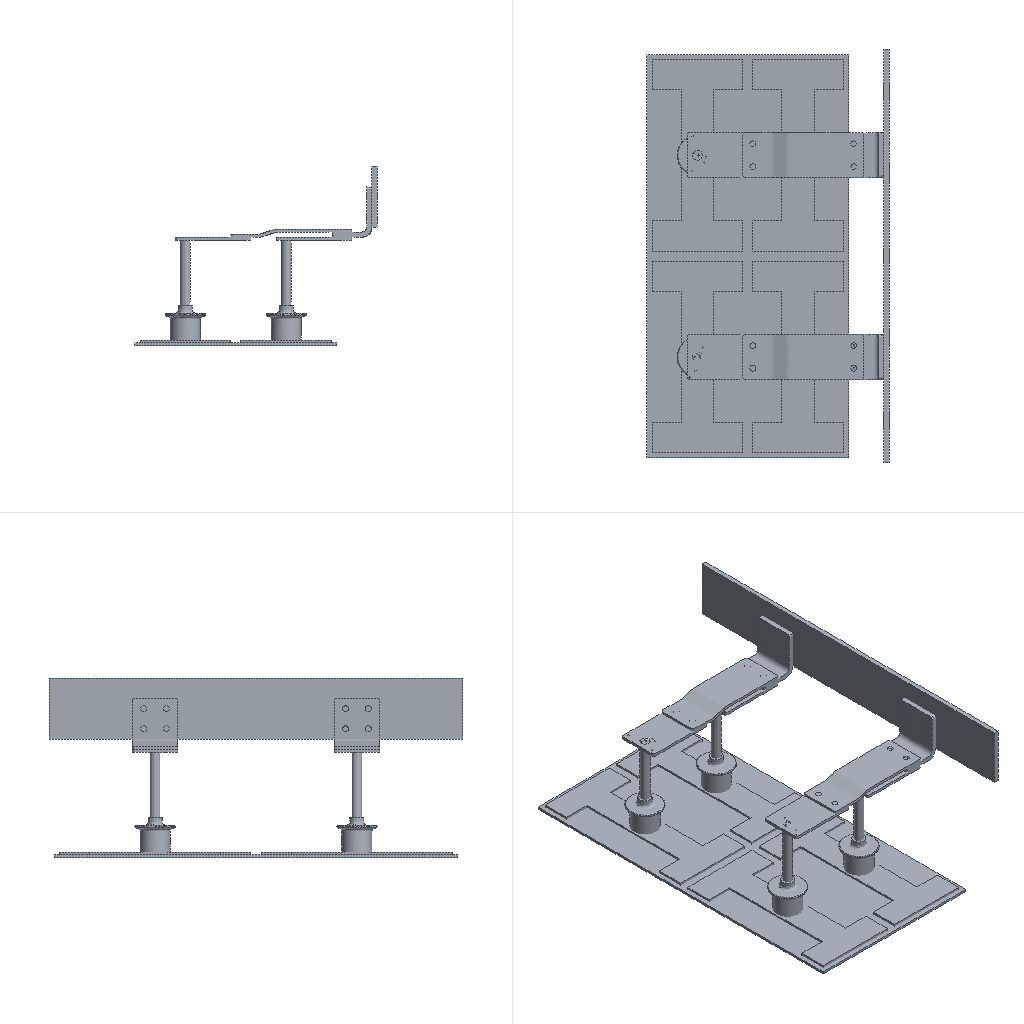Simulation study | ansys workbench
Set-up summary:
category,name,step,type,value,unit,region
solver,ansys_mapdl
solver,version,,,25.1
units,MKS,,stated
analysis,deck,,static,static
load_step,requested,,,1
analysis,nlgeom,,,False
mesh,nodes,,,1129327
mesh,elements,,,564596
element_type,ANSYS 226 (type 1),,coupled_solid,71556
element_type,ANSYS 226 (type 2),,coupled_solid,8280
element_type,ANSYS 226 (type 3),,coupled_solid,8280
element_type,ANSYS 226 (type 4),,coupled_solid,4563
element_type,ANSYS 226 (type 5),,coupled_solid,4530
element_type,ANSYS 226 (type 6),,coupled_solid,4644
element_type,ANSYS 227 (type 7),,coupled_solid,9584
element_type,ANSYS 226 (type 8),,coupled_solid,5940
element_type,ANSYS 227 (type 9),,coupled_solid,9554
element_type,ANSYS 227 (type 10),,coupled_solid,8027
element_type,ANSYS 227 (type 11),,coupled_solid,8037
element_type,ANSYS 226 (type 12),,coupled_solid,130
element_type,ANSYS 226 (type 13),,coupled_solid,130
element_type,ANSYS 226 (type 14),,coupled_solid,120
element_type,ANSYS 226 (type 15),,coupled_solid,120
element_type,ANSYS 226 (type 16),,coupled_solid,8280
element_type,ANSYS 226 (type 17),,coupled_solid,8280
element_type,ANSYS 226 (type 18),,coupled_solid,4527
element_type,ANSYS 226 (type 19),,coupled_solid,4545
element_type,ANSYS 226 (type 20),,coupled_solid,4644
element_type,ANSYS 227 (type 21),,coupled_solid,9619
element_type,ANSYS 226 (type 22),,coupled_solid,5940
element_type,ANSYS 227 (type 23),,coupled_solid,9514
element_type,ANSYS 227 (type 24),,coupled_solid,8103
element_type,ANSYS 227 (type 25),,coupled_solid,8073
element_type,ANSYS 226 (type 26),,coupled_solid,208
element_type,ANSYS 226 (type 27),,coupled_solid,208
element_type,ANSYS 226 (type 28),,coupled_solid,208
element_type,ANSYS 226 (type 29),,coupled_solid,208
element_type,ANSYS 226 (type 30),,coupled_solid,168
element_type,ANSYS 226 (type 31),,coupled_solid,168
element_type,ANSYS 226 (type 32),,coupled_solid,168
element_type,ANSYS 226 (type 33),,coupled_solid,168
element_type,ANSYS 226 (type 34),,coupled_solid,182
element_type,ANSYS 226 (type 35),,coupled_solid,182
element_type,ANSYS 226 (type 36),,coupled_solid,182
element_type,ANSYS 226 (type 37),,coupled_solid,182
element_type,ANSYS 226 (type 38),,coupled_solid,43852
element_type,ANSYS 174 (type 39),,contact,9539
element_type,ANSYS 170 (type 40),,target,9539
element_type,ANSYS 174 (type 41),,contact,9539
element_type,ANSYS 170 (type 42),,target,9539
element_type,ANSYS 174 (type 43),,contact,9539
element_type,ANSYS 170 (type 44),,target,9539
element_type,ANSYS 174 (type 45),,contact,9539
element_type,ANSYS 170 (type 46),,target,9539
element_type,ANSYS 174 (type 47),,contact,677
element_type,ANSYS 170 (type 48),,target,677
element_type,ANSYS 174 (type 49),,contact,677
element_type,ANSYS 170 (type 50),,target,677
element_type,ANSYS 174 (type 51),,contact,151
element_type,ANSYS 170 (type 52),,target,151
element_type,ANSYS 174 (type 53),,contact,812
element_type,ANSYS 170 (type 54),,target,812
element_type,ANSYS 174 (type 55),,contact,109
element_type,ANSYS 170 (type 56),,target,109
element_type,ANSYS 174 (type 57),,contact,109
element_type,ANSYS 170 (type 58),,target,109
element_type,ANSYS 174 (type 59),,contact,151
element_type,ANSYS 170 (type 60),,target,151
element_type,ANSYS 174 (type 61),,contact,805
element_type,ANSYS 170 (type 62),,target,805
element_type,ANSYS 174 (type 63),,contact,109
element_type,ANSYS 170 (type 64),,target,109
element_type,ANSYS 174 (type 65),,contact,109
element_type,ANSYS 170 (type 66),,target,109
element_type,ANSYS 174 (type 67),,contact,661
element_type,ANSYS 170 (type 68),,target,661
element_type,ANSYS 174 (type 69),,contact,685
element_type,ANSYS 170 (type 70),,target,685
element_type,ANSYS 174 (type 71),,contact,116
element_type,ANSYS 170 (type 72),,target,116
element_type,ANSYS 174 (type 73),,contact,108
element_type,ANSYS 170 (type 74),,target,108
element_type,ANSYS 174 (type 75),,contact,697
element_type,ANSYS 170 (type 76),,target,697
element_type,ANSYS 174 (type 77),,contact,110
element_type,ANSYS 170 (type 78),,target,110
element_type,ANSYS 174 (type 79),,contact,112
element_type,ANSYS 170 (type 80),,target,112
element_type,ANSYS 174 (type 81),,contact,108
element_type,ANSYS 170 (type 82),,target,108
element_type,ANSYS 174 (type 83),,contact,116
element_type,ANSYS 170 (type 84),,target,116
element_type,ANSYS 174 (type 85),,contact,690
element_type,ANSYS 170 (type 86),,target,690
element_type,ANSYS 174 (type 87),,contact,112
element_type,ANSYS 170 (type 88),,target,112
element_type,ANSYS 174 (type 89),,contact,110
element_type,ANSYS 170 (type 90),,target,110
element_type,ANSYS 174 (type 91),,contact,677
element_type,ANSYS 170 (type 92),,target,677
element_type,ANSYS 174 (type 93),,contact,677
element_type,ANSYS 170 (type 94),,target,677
element_type,ANSYS 174 (type 95),,contact,151
element_type,ANSYS 170 (type 96),,target,151
element_type,ANSYS 174 (type 97),,contact,822
element_type,ANSYS 170 (type 98),,target,822
element_type,ANSYS 174 (type 99),,contact,109
element_type,ANSYS 170 (type 100),,target,109
element_type,ANSYS 174 (type 101),,contact,109
element_type,ANSYS 170 (type 102),,target,109
element_type,ANSYS 174 (type 103),,contact,151
element_type,ANSYS 170 (type 104),,target,151
element_type,ANSYS 174 (type 105),,contact,815
element_type,ANSYS 170 (type 106),,target,815
element_type,ANSYS 174 (type 107),,contact,109
element_type,ANSYS 170 (type 108),,target,109
element_type,ANSYS 174 (type 109),,contact,109
element_type,ANSYS 170 (type 110),,target,109
element_type,ANSYS 174 (type 111),,contact,685
element_type,ANSYS 170 (type 112),,target,685
element_type,ANSYS 174 (type 113),,contact,669
element_type,ANSYS 170 (type 114),,target,669
element_type,ANSYS 174 (type 115),,contact,190
element_type,ANSYS 170 (type 116),,target,190
element_type,ANSYS 174 (type 117),,contact,190
element_type,ANSYS 170 (type 118),,target,190
element_type,ANSYS 174 (type 119),,contact,162
element_type,ANSYS 170 (type 120),,target,162
element_type,ANSYS 174 (type 121),,contact,162
element_type,ANSYS 170 (type 122),,target,162
element_type,ANSYS 174 (type 123),,contact,162
element_type,ANSYS 170 (type 124),,target,162
element_type,ANSYS 174 (type 125),,contact,162
element_type,ANSYS 170 (type 126),,target,162
element_type,ANSYS 174 (type 127),,contact,1548
element_type,ANSYS 170 (type 128),,target,1548
element_type,ANSYS 174 (type 129),,contact,190
element_type,ANSYS 170 (type 130),,target,190
element_type,ANSYS 174 (type 131),,contact,190
element_type,ANSYS 170 (type 132),,target,190
element_type,ANSYS 174 (type 133),,contact,162
element_type,ANSYS 170 (type 134),,target,162
element_type,ANSYS 174 (type 135),,contact,162
element_type,ANSYS 170 (type 136),,target,162
element_type,ANSYS 174 (type 137),,contact,162
element_type,ANSYS 170 (type 138),,target,162
element_type,ANSYS 174 (type 139),,contact,162
element_type,ANSYS 170 (type 140),,target,162
element_type,ANSYS 174 (type 141),,contact,1613
element_type,ANSYS 170 (type 142),,target,1613
element_type,ANSYS 174 (type 143),,contact,136
element_type,ANSYS 170 (type 144),,target,136
element_type,ANSYS 174 (type 145),,contact,136
element_type,ANSYS 170 (type 146),,target,136
element_type,ANSYS 174 (type 147),,contact,136
element_type,ANSYS 170 (type 148),,target,136
element_type,ANSYS 174 (type 149),,contact,136
element_type,ANSYS 170 (type 150),,target,136
element_type,ANSYS 174 (type 151),,contact,136
element_type,ANSYS 170 (type 152),,target,136
element_type,ANSYS 174 (type 153),,contact,136
element_type,ANSYS 170 (type 154),,target,136
element_type,ANSYS 174 (type 155),,contact,136
element_type,ANSYS 170 (type 156),,target,136
element_type,ANSYS 174 (type 157),,contact,136
element_type,ANSYS 170 (type 158),,target,136
element_type,ANSYS 152 (type 159),,surface,153958
element_type,ANSYS 152 (type 160),,surface,35778
load,load commands in deck,,count,3
bc,support commands in deck,,count,3
named_set,_CM326,,component
named_set,_ELMISC,,component
material,1,,in results
material,2,,in results
material,3,,in results
material,4,,in results
material,5,,in results
material,6,,in results
material,7,,in results
material,8,,in results
material,9,,in results
material,10,,in results
material,11,,in results
material,12,,in results
material,13,,in results
material,14,,in results
material,15,,in results
material,16,,in results
material,17,,in results
material,18,,in results
material,19,,in results
material,20,,in results
material,21,,in results
material,22,,in results
material,23,,in results
material,24,,in results
material,25,,in results
material,26,,in results
material,27,,in results
material,28,,in results
material,29,,in results
material,30,,in results
material,31,,in results
material,32,,in results
material,33,,in results
material,34,,in results
material,35,,in results
material,36,,in results
material,37,,in results
material,38,,in results
check,setup vs results,,match,189736 surface effect element(s) are not in the reader's mesh and were not compared
Ansys APDL input file, long lists of numbers shortened:
/batch
/config,noeldb,1     ! force off writing results to database
*get,_wallstrt,active,,time,wall
! ANSYS input file written by Workbench version 2025 R1
! File used for geometry attach: D:\02_WXG\007-CAE\00_CAE Examples_SelfSim\017_Thermal_Mechanical\002_Busbar_TM\Busbar_TM_files\dp0\Geom\DM\Geom.scdocx
/title,Busbar_TM--Steady-State Thermal-Electric Conduction (B5)
! ****** Begin Custom Load Command Snippet ******
/COM, ACT Extensions:
/COM,     LSDYNA, 2025.1
/COM,/COM,     ANSYSMotion, 2025.1
/COM,
! ****** End   Custom Load Command Snippet ******
*DIM,_wb_ProjectScratch_dir,string,248
_wb_ProjectScratch_dir(1) = 'D:\02_WXG\007-CAE\00_CAE Examples_SelfSim\017_Thermal_Mechanical\002_Busbar_TM\_ProjectScratch\ScrBBAA\'
*DIM,_wb_SolverFiles_dir,string,248
_wb_SolverFiles_dir(1) = 'D:\02_WXG\007-CAE\00_CAE Examples_SelfSim\017_Thermal_Mechanical\002_Busbar_TM\Busbar_TM_files\dp0\SYS\MECH\'
*DIM,_wb_userfiles_dir,string,248
_wb_userfiles_dir(1) = 'D:\02_WXG\007-CAE\00_CAE Examples_SelfSim\017_Thermal_Mechanical\002_Busbar_TM\Busbar_TM_files\user_files\'
/com,--- Data in consistent MKS units. See Solving Units in the help system for more information.
/units,MKS
/nopr
/wb,file,start              !  signify a WB generated input file
/prep7
! Turn off shape checking because checks already performed inside WB mesher.
! See help system for more information.
SHPP,OFF,,NOWARN
/nolist
etcon,set             ! allow ANSYS to choose best KEYOP's for 180x elements, resets any applicable keyopt to MAPDL defaults
/com,*********** Nodes for the whole assembly ***********
nblock,3,,1242259
(1i9,3e20.9e3)
        1     1.970149254E-01     3.970037453E-01     2.500000000E-03
! (1129326 more lines like these left out)
-1
/wb,elem,start            !  set before creation of elements
/com,*********** Elements for Body 1 'id2\id2' ***********
et,1,226,110
eblock,19,solid,,71556
(19i9)
        1        1        1        1        0        0        0        0       20        0        1        1   107207   107205   107069    70756   107738   107206   107070
! (143111 more lines like these left out)
-1
/com,*********** Elements for Body 2 'id5\id5' ***********
et,2,226,110
eblock,19,solid,,8280
(19i9)
        2        2        2        2        0        0        0        0       20        0    71557   396772   409544   409583   409584   404599   409581   409582   409603
! (16559 more lines like these left out)
-1
/com,*********** Elements for Body 3 'id8\id8' ***********
et,3,226,110
eblock,19,solid,,8280
(19i9)
        3        3        3        3        0        0        0        0       20        0    79837   444133   456603   456584   456545   451960   456622   456583   456564
! (16559 more lines like these left out)
-1
/com,*********** Elements for Body 4 'id11\id11' ***********
et,4,226,110
eblock,19,solid,,4563
(19i9)
        4        4        4        4        0        0        0        0       20        0    88117   491552   494214   491642   494208   495700   494369   495655   494372
! (9125 more lines like these left out)
-1
/com,*********** Elements for Body 5 'id14\id14' ***********
et,5,226,110
eblock,19,solid,,4530
(19i9)
        5        5        5        5        0        0        0        0       20        0    92680   516018   516020   516338   518180   519302   519301   519142   518221
! (9059 more lines like these left out)
-1
! (26 more sections like these left out)
/com,*********** Elements for Body 32 'id95\COMSOL_BodyMinVertex$925' ***********
et,32,226,110
eblock,19,solid,,168
(19i9)
       32       32       32       32        0        0        0        0       20        0   216189   910258   910294   910300   910306   910383   910377   910376   910375
! (335 more lines like these left out)
-1
! (6 more sections like these left out)
/wb,elem,end               !  done creating elements
/com,*********** Send User Defined Coordinate System(s) ***********
csys,0
toffst,273.15,      ! Temperature offset from absolute zero
/com,*********** Set Reference Temperature ***********
tref,35.
/wb,mat,start              !  starting to send materials
/com,*********** Send Materials ***********
MP,KXX,1,7.5,	! W m^-1 C^-1
MP,RSVX,1,1.35007425408398e-06,	! kg m^3 A^-2 s^-3
MP,KXX,2,7.5,	! W m^-1 C^-1
! (110 more lines like these left out)
/wb,mat,end                !  done sending materials
!************************* Model Summary ********************
!id2\id2,	Titanium,	matid,	1
!id5\id5,	Titanium,	matid,	2
!id8\id8,	Titanium,	matid,	3
! (37 more lines like these left out)
*get,_xmin,node,,mnloc,x
*get,_ymin,node,,mnloc,y
*get,_zmin,node,,mnloc,z
*get,_xmax,node,,mxloc,x
*get,_ymax,node,,mxloc,y
*get,_zmax,node,,mxloc,z
_ASMDIAG=(_xmax-_xmin)*(_xmax-_xmin)+(_ymax-_ymin)*(_ymax-_ymin)+(_zmax-_zmin)*(_zmax-_zmin)
_ASMDIAG=SQRT(_ASMDIAG)
/wb,contact,start          !  starting to send contact
/com,*********** Create Contact "Contact Region" ***********
/com,            Real Constant Set For Above Contact Is 40 & 39
*set,tid,40
*set,cid,39
r,tid
r,cid
et,tid,170
et,cid,174
eblock,10,,,5399
(15i9)
   450841       40       40       40        0    52866    52733    52734    52867   285425   285424   285427   285691
! (5398 more lines like these left out)
-1
eblock,10,,,5399
(15i9)
   456240       39       39       39        0    52866    52733    52734    52867   285425   285424   285427   285691
! (5398 more lines like these left out)
-1
eblock,10,,,4140
(15i9)
   461639       39       40       39        0   409603   404599   409581   409582   433809   433808   443693   443695
! (4139 more lines like these left out)
-1
eblock,10,,,4140
(15i9)
   465779       40       39       40        0   409603   404599   409581   409582   433809   433808   443693   443695
! (4139 more lines like these left out)
-1
keyo,cid,8,2               ! auto create asymmetric contact (from Program Controlled setting)
keyo,cid,10,0              ! adjust contact stiffness each NR iteration (from Program Controlled setting)
keyo,cid,12,5              ! bonded always
keyo,cid,18,1              ! small sliding turned on by application
keyo,cid,2,0               ! augmented Lagrange (from Program Controlled setting)
keyo,cid,4,0               ! on Gauss point (from Program Controlled setting)
keyo,cid,9,1               ! ignore initial gaps/penetration
keyo,cid,7,0               ! No Prediction
rmod,tid,3,10.      ! FKN
rmod,tid,5,0.       ! ICONT
rmod,tid,6,0.       ! PINB
rmod,tid,10,0.      ! CNOF
rmod,tid,12,0.      ! FKT
rmod,tid,36,139     ! WB DSID
rmod,cid,3,10.      ! FKN
rmod,cid,5,0.       ! ICONT
rmod,cid,6,0.       ! PINB
rmod,cid,10,0.      ! CNOF
rmod,cid,12,0.      ! FKT
rmod,cid,36,139     ! WB DSID
*set,_maxkxx,4000000.
rmod,cid,14,_maxkxx/_ASMDIAG         ! TCC, Divide by Length since Traction Based
rmod,tid,14,_maxkxx/_ASMDIAG      ! TCC, Divide by Length since Traction Based
*set,_maxCond,599799999999.999
rmod,cid,19,_maxCond/_ASMDIAG      ! ECC
rmod,tid,19,_maxCond/_ASMDIAG     ! ECC
keyo,cid,1,4     ! Thermo-Electric contact
/com,*********** Create Contact "Contact Region 2" ***********
/com,            Real Constant Set For Above Contact Is 42 & 41
*set,tid,42
*set,cid,41
r,tid
r,cid
et,tid,170
et,cid,174
eblock,10,,,5399
(15i9)
   469919       42       42       42        0    70688    70555    70556    70689   321203   321202   321205   321469
! (5398 more lines like these left out)
-1
eblock,10,,,5399
(15i9)
   475318       41       41       41        0    70688    70555    70556    70689   321203   321202   321205   321469
! (5398 more lines like these left out)
-1
eblock,10,,,4140
(15i9)
   480717       41       42       41        0   456564   451960   456622   456583   481169   481170   490516   490497
! (4139 more lines like these left out)
-1
eblock,10,,,4140
(15i9)
   484857       42       41       42        0   456564   451960   456622   456583   481169   481170   490516   490497
! (4139 more lines like these left out)
-1
keyo,cid,8,2               ! auto create asymmetric contact (from Program Controlled setting)
keyo,cid,10,0              ! adjust contact stiffness each NR iteration (from Program Controlled setting)
keyo,cid,12,5              ! bonded always
keyo,cid,18,1              ! small sliding turned on by application
keyo,cid,2,0               ! augmented Lagrange (from Program Controlled setting)
keyo,cid,4,0               ! on Gauss point (from Program Controlled setting)
keyo,cid,9,1               ! ignore initial gaps/penetration
keyo,cid,7,0               ! No Prediction
rmod,tid,3,10.      ! FKN
rmod,tid,5,0.       ! ICONT
rmod,tid,6,0.       ! PINB
rmod,tid,10,0.      ! CNOF
rmod,tid,12,0.      ! FKT
rmod,tid,36,142     ! WB DSID
rmod,cid,3,10.      ! FKN
rmod,cid,5,0.       ! ICONT
rmod,cid,6,0.       ! PINB
rmod,cid,10,0.      ! CNOF
rmod,cid,12,0.      ! FKT
rmod,cid,36,142     ! WB DSID
*set,_maxkxx,4000000.
rmod,cid,14,_maxkxx/_ASMDIAG         ! TCC, Divide by Length since Traction Based
rmod,tid,14,_maxkxx/_ASMDIAG      ! TCC, Divide by Length since Traction Based
*set,_maxCond,599799999999.999
rmod,cid,19,_maxCond/_ASMDIAG      ! ECC
rmod,tid,19,_maxCond/_ASMDIAG     ! ECC
keyo,cid,1,4     ! Thermo-Electric contact
/com,*********** Create Contact "Contact Region 3" ***********
/com,            Real Constant Set For Above Contact Is 44 & 43
*set,tid,44
*set,cid,43
r,tid
r,cid
et,tid,170
et,cid,174
eblock,10,,,5399
(15i9)
   488997       44       44       44        0    52933    52800    52801    52934   285559   285558   285560   285825
! (5398 more lines like these left out)
-1
eblock,10,,,5399
(15i9)
   494396       43       43       43        0    52933    52800    52801    52934   285559   285558   285560   285825
! (5398 more lines like these left out)
-1
eblock,10,,,4140
(15i9)
   499795       43       44       43        0   665080   660076   665058   665059   689286   689285   699170   699172
! (4139 more lines like these left out)
-1
eblock,10,,,4140
(15i9)
   503935       44       43       44        0   665080   660076   665058   665059   689286   689285   699170   699172
! (4139 more lines like these left out)
-1
keyo,cid,8,2               ! auto create asymmetric contact (from Program Controlled setting)
keyo,cid,10,0              ! adjust contact stiffness each NR iteration (from Program Controlled setting)
keyo,cid,12,5              ! bonded always
keyo,cid,18,1              ! small sliding turned on by application
keyo,cid,2,0               ! augmented Lagrange (from Program Controlled setting)
keyo,cid,4,0               ! on Gauss point (from Program Controlled setting)
keyo,cid,9,1               ! ignore initial gaps/penetration
keyo,cid,7,0               ! No Prediction
rmod,tid,3,10.      ! FKN
rmod,tid,5,0.       ! ICONT
rmod,tid,6,0.       ! PINB
rmod,tid,10,0.      ! CNOF
rmod,tid,12,0.      ! FKT
rmod,tid,36,145     ! WB DSID
rmod,cid,3,10.      ! FKN
rmod,cid,5,0.       ! ICONT
rmod,cid,6,0.       ! PINB
rmod,cid,10,0.      ! CNOF
rmod,cid,12,0.      ! FKT
rmod,cid,36,145     ! WB DSID
*set,_maxkxx,4000000.
rmod,cid,14,_maxkxx/_ASMDIAG         ! TCC, Divide by Length since Traction Based
rmod,tid,14,_maxkxx/_ASMDIAG      ! TCC, Divide by Length since Traction Based
*set,_maxCond,599799999999.999
rmod,cid,19,_maxCond/_ASMDIAG      ! ECC
rmod,tid,19,_maxCond/_ASMDIAG     ! ECC
keyo,cid,1,4     ! Thermo-Electric contact
/com,*********** Create Contact "Contact Region 4" ***********
/com,            Real Constant Set For Above Contact Is 46 & 45
*set,tid,46
*set,cid,45
r,tid
r,cid
et,tid,170
et,cid,174
eblock,10,,,5399
(15i9)
   508075       46       46       46        0    70755    70622    70623    70756   321337   321336   321338   321603
! (5398 more lines like these left out)
-1
eblock,10,,,5399
(15i9)
   513474       45       45       45        0    70755    70622    70623    70756   321337   321336   321338   321603
! (5398 more lines like these left out)
-1
eblock,10,,,4140
(15i9)
   518873       45       46       45        0   711352   707438   711804   711805   736650   736651   745606   744702
! (4139 more lines like these left out)
-1
eblock,10,,,4140
(15i9)
   523013       46       45       46        0   711352   707438   711804   711805   736650   736651   745606   744702
! (4139 more lines like these left out)
-1
keyo,cid,8,2               ! auto create asymmetric contact (from Program Controlled setting)
keyo,cid,10,0              ! adjust contact stiffness each NR iteration (from Program Controlled setting)
keyo,cid,12,5              ! bonded always
keyo,cid,18,1              ! small sliding turned on by application
keyo,cid,2,0               ! augmented Lagrange (from Program Controlled setting)
keyo,cid,4,0               ! on Gauss point (from Program Controlled setting)
keyo,cid,9,1               ! ignore initial gaps/penetration
keyo,cid,7,0               ! No Prediction
rmod,tid,3,10.      ! FKN
rmod,tid,5,0.       ! ICONT
rmod,tid,6,0.       ! PINB
rmod,tid,10,0.      ! CNOF
rmod,tid,12,0.      ! FKT
rmod,tid,36,148     ! WB DSID
rmod,cid,3,10.      ! FKN
rmod,cid,5,0.       ! ICONT
rmod,cid,6,0.       ! PINB
rmod,cid,10,0.      ! CNOF
rmod,cid,12,0.      ! FKT
rmod,cid,36,148     ! WB DSID
*set,_maxkxx,4000000.
rmod,cid,14,_maxkxx/_ASMDIAG         ! TCC, Divide by Length since Traction Based
rmod,tid,14,_maxkxx/_ASMDIAG      ! TCC, Divide by Length since Traction Based
*set,_maxCond,599799999999.999
rmod,cid,19,_maxCond/_ASMDIAG      ! ECC
rmod,tid,19,_maxCond/_ASMDIAG     ! ECC
keyo,cid,1,4     ! Thermo-Electric contact
/com,*********** Create Contact "Contact Region 5" ***********
/com,            Real Constant Set For Above Contact Is 48 & 47
*set,tid,48
*set,cid,47
r,tid
r,cid
et,tid,170
et,cid,174
eblock,10,,,456
(15i9)
   527153       48       48       48        0   408830   406367   406348   408831   437496   437456   437457   442497
! (455 more lines like these left out)
-1
eblock,10,,,456
(15i9)
   527609       47       47       47        0   408830   406367   406348   408831   437496   437456   437457   442497
! (455 more lines like these left out)
-1
eblock,10,,,221
(15i9)
   528065       47       48       47        0   561363   561399   561377   561377   573141   573233   561377   573140
! (220 more lines like these left out)
-1
eblock,10,,,221
(15i9)
   528286       48       47       48        0   561363   561399   561377   561377   573141   573233   561377   573140
! (220 more lines like these left out)
-1
keyo,cid,8,2               ! auto create asymmetric contact (from Program Controlled setting)
keyo,cid,10,0              ! adjust contact stiffness each NR iteration (from Program Controlled setting)
keyo,cid,12,5              ! bonded always
keyo,cid,18,1              ! small sliding turned on by application
keyo,cid,2,0               ! augmented Lagrange (from Program Controlled setting)
keyo,cid,4,0               ! on Gauss point (from Program Controlled setting)
keyo,cid,9,1               ! ignore initial gaps/penetration
keyo,cid,7,0               ! No Prediction
rmod,tid,3,10.      ! FKN
rmod,tid,5,0.       ! ICONT
rmod,tid,6,0.       ! PINB
rmod,tid,10,0.      ! CNOF
rmod,tid,12,0.      ! FKT
rmod,tid,36,151     ! WB DSID
rmod,cid,3,10.      ! FKN
rmod,cid,5,0.       ! ICONT
rmod,cid,6,0.       ! PINB
rmod,cid,10,0.      ! CNOF
rmod,cid,12,0.      ! FKT
rmod,cid,36,151     ! WB DSID
*set,_maxkxx,4000000.
rmod,cid,14,_maxkxx/_ASMDIAG         ! TCC, Divide by Length since Traction Based
rmod,tid,14,_maxkxx/_ASMDIAG      ! TCC, Divide by Length since Traction Based
*set,_maxCond,599799999999.999
rmod,cid,19,_maxCond/_ASMDIAG      ! ECC
rmod,tid,19,_maxCond/_ASMDIAG     ! ECC
keyo,cid,1,4     ! Thermo-Electric contact
! (55 more sections like these left out)
/wb,contact,end            !  done creating contacts
/golist
/wb,load,start             !  starting to send loads
/com,*********** Create Voltage "Voltage" ***********
CMBLOCK,_CM326  ,NODE,     1138
(8i10)
    969333    969334    969335    969336    969337    969338    969339    969340
! (142 more lines like these left out)
/com,*********** Create Current ***********
fcum,add                   ! add nodal forces up (needed in case have loads on the same edge,vertex)
fcum                       ! reset default on fcum command since done sending WB F loads
/com,*********** Create "Convection" ***********
et,159,152
eblock,10,,,153958
(15i9)
   564597      159      159      159        0   107202   106937   107203   107204   394367   394368   394767   394766
! (153957 more lines like these left out)
-1
esel,s,type,,159
keyop,159,8,2
keyop,159,13,0
/com,*********** Create "Convection 2" ***********
et,160,152
eblock,10,,,35778
(15i9)
   718555      160      160      160        0   106535    70757   106935   106936   321609   321610   394363   393564
! (35777 more lines like these left out)
-1
esel,s,type,,160
keyop,160,8,2
keyop,160,13,0
esel,all
/gst,on,on
fini
*get,_numnode,node,0,count
*get,_numelem,elem,0,count
*get, _MAXELEMNUM, elem, 0, NUM, MAX
*get, _MAXNODENUM, node, 0, NUM, MAX
*get, _MAXELEMTYPE, etyp, 0, NUM, MAX
*get, _MAXREALCONST, rcon, 0, NUM, MAX
/go
/wb,load,end               !  done creating loads
/com,--- Number of total nodes = %_numnode%
/com,--- Number of contact elements = 303492
/com,--- Number of spring elements = 0
/com,--- Number of bearing elements = 0
/com,--- Number of solid elements = 261104
/com,--- Number of condensed parts = 0
/com,--- Number of total elements = %_numelem%
*get,_wallbsol,active,,time,wall
/com,****************************************************************************
/com,*************************    SOLUTION       ********************************
/com,****************************************************************************
/solu
antype,0                   ! static analysis
!eqsl,sparse               ! using sparse solver which is default so no eqsl command needed
cntr,print,1               ! print out contact info and also make no initial contact an error
/com,****************************************************
/com,******************* SOLVE FOR LS 1 OF 1****************
d,_CM326,volt,0.
nsel,all
f,70757,amps,2560.
ce,next,0.,70757,volt,-1.,70758,volt,1.
ce,next,0.,70757,volt,-1.,70759,volt,1.
! (108134 more lines like these left out)
/nopr
/gopr
esel,s,type,,159
nsle
sf,all,conv,5.,35.
esel,s,type,,160
nsle
sf,all,conv,3000.,100.
nsel,all
esel,all
autots,on
nsub,1,10,1
time,1.
outres,erase
outres,all,none
outres,nsol,all
outres,rsol,all
outres,eangl,all
outres,veng,all
outres,fflux,all
outres,fgrad,all
outres,eheat,all,
outres,cont,all,
/nopr
esel,s,type,,159
esel,a,type,,160
cm,_elmisc,elem
esel,all
/gopr
outres,misc,all,_elmisc
cnvtol,heat,,1.e-003,,1.e-006 ! Program Controlled. Set MINREF equivalent of 1e-6 Watts
cnvtol,amps,,1.e-003,,1.e-006 ! Program Controlled. Set MINREF equivalent of 1e-6 A
neqit,1000
! *********** WB SOLVE COMMAND ***********
! check interactive state
*get,ANSINTER_,active,,int
*if,ANSINTER_,ne,0,then
/eof
*endif
solve
/com *************** Write FE CONNECTORS *********
CEWRITE,file,ce,,INTE
/com,****************************************************
/com,*************** FINISHED SOLVE FOR LS 1 *************
*get,_wallasol,active,,time,wall
/post1
xmlo,ENCODING,ISO-8859-1
xmlo,parm
/xml,parm,xml
fini
/gopr
*get,_walldone,active,,time,wall
_preptime=(_wallbsol-_wallstrt)*3600
_solvtime=(_wallasol-_wallbsol)*3600
_posttime=(_walldone-_wallasol)*3600
_totaltim=(_walldone-_wallstrt)*3600
*get,_dlbratio,active,0,solu,dlbr
*get,_combtime,active,0,solu,comb
*get,_ssmode,active,0,solu,ssmm
*get,_ndofs,active,0,solu,ndof
/com,--- Total number of nodes = %_numnode%
/com,--- Total number of elements = %_numelem%
/com,--- Element load balance ratio = %_dlbratio%
/com,--- Time to combine distributed files = %_combtime%
/com,--- Sparse memory mode = %_ssmode%
/com,--- Number of DOF = %_ndofs%
/wb,file,end               ! done with WB generated input
Results summary:
result,analysis,,,static
result,last_loadstep,,,1
result,primary field,,,temperature